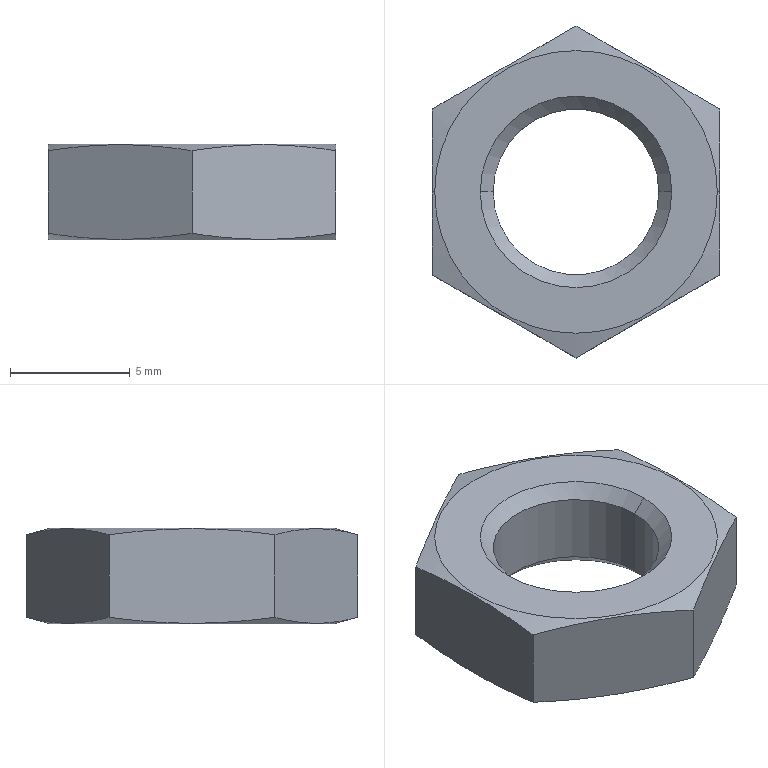Part | SolidWorks | features BaseBody 1 | 1 solid | 18 faces | box 12 x 13.856 x 4 mm | volume 339.344 mm3 | cone 8 | plane 8 | cylinder 2 | commonest cylinder face diameters 6.917 x2
STEP:
#1=CARTESIAN_POINT('',(3.459,0.,0.5415));
#2=VERTEX_POINT('',#1);
#3=CARTESIAN_POINT('',(-3.459,0.,0.5415));
#4=VERTEX_POINT('',#3);
#5=CARTESIAN_POINT('',(0.,0.,0.5415));
#6=DIRECTION('',(0.,0.,-1.));
#7=DIRECTION('',(-1.,0.,0.));
#8=AXIS2_PLACEMENT_3D('',#5,#6,#7);
#9=CIRCLE('',#8,3.459);
#10=EDGE_CURVE('',#2,#4,#9,.T.);
#11=ORIENTED_EDGE('',*,*,#10,.F.);
#12=CARTESIAN_POINT('',(4.,0.,0.));
#13=VERTEX_POINT('',#12);
#14=CARTESIAN_POINT('',(3.459,0.,0.5415));
#15=DIRECTION('',(0.7071,0.,-0.7071));
#16=VECTOR('',#15,1000.);
#17=LINE('',#14,#16);
#18=EDGE_CURVE('',#2,#13,#17,.T.);
#19=ORIENTED_EDGE('',*,*,#18,.T.);
#20=CARTESIAN_POINT('',(-4.,0.,0.));
#21=VERTEX_POINT('',#20);
#22=CARTESIAN_POINT('',(0.,0.,0.));
#23=DIRECTION('',(0.,0.,-1.));
#24=DIRECTION('',(-1.,0.,0.));
#25=AXIS2_PLACEMENT_3D('',#22,#23,#24);
#26=CIRCLE('',#25,4.);
#27=EDGE_CURVE('',#13,#21,#26,.T.);
#28=ORIENTED_EDGE('',*,*,#27,.T.);
#29=CARTESIAN_POINT('',(-3.459,0.,0.5415));
#30=DIRECTION('',(-0.7071,0.,-0.7071));
#31=VECTOR('',#30,1000.);
#32=LINE('',#29,#31);
#33=EDGE_CURVE('',#4,#21,#32,.T.);
#34=ORIENTED_EDGE('',*,*,#33,.F.);
#35=EDGE_LOOP('',(#11,#19,#28,#34));
#36=FACE_OUTER_BOUND('',#35,.T.);
#37=CARTESIAN_POINT('',(0.,0.,0.5415));
#38=DIRECTION('',(0.,0.,-1.));
#39=DIRECTION('',(-1.,0.,0.));
#40=AXIS2_PLACEMENT_3D('',#37,#38,#39);
#41=CONICAL_SURFACE('',#40,3.459,0.7854);
#42=ADVANCED_FACE('',(#36),#41,.F.);
#43=CARTESIAN_POINT('',(3.459,0.,3.459));
#44=VERTEX_POINT('',#43);
#45=CARTESIAN_POINT('',(-3.459,0.,3.459));
#46=VERTEX_POINT('',#45);
#47=CARTESIAN_POINT('',(0.,0.,3.459));
#48=DIRECTION('',(0.,0.,-1.));
#49=DIRECTION('',(-1.,0.,0.));
#50=AXIS2_PLACEMENT_3D('',#47,#48,#49);
#51=CIRCLE('',#50,3.459);
#52=EDGE_CURVE('',#44,#46,#51,.T.);
#53=ORIENTED_EDGE('',*,*,#52,.F.);
#54=CARTESIAN_POINT('',(3.459,0.,0.));
#55=DIRECTION('',(0.,0.,-1.));
#56=VECTOR('',#55,1000.);
#57=LINE('',#54,#56);
#58=EDGE_CURVE('',#44,#2,#57,.T.);
#59=ORIENTED_EDGE('',*,*,#58,.T.);
#60=ORIENTED_EDGE('',*,*,#10,.T.);
#61=CARTESIAN_POINT('',(-3.459,0.,0.));
#62=DIRECTION('',(0.,0.,-1.));
#63=VECTOR('',#62,1000.);
#64=LINE('',#61,#63);
#65=EDGE_CURVE('',#46,#4,#64,.T.);
#66=ORIENTED_EDGE('',*,*,#65,.F.);
#67=EDGE_LOOP('',(#53,#59,#60,#66));
#68=FACE_OUTER_BOUND('',#67,.T.);
#69=CARTESIAN_POINT('',(0.,0.,0.));
#70=DIRECTION('',(0.,0.,-1.));
#71=DIRECTION('',(-1.,0.,0.));
#72=AXIS2_PLACEMENT_3D('',#69,#70,#71);
#73=CYLINDRICAL_SURFACE('',#72,3.459);
#74=ADVANCED_FACE('',(#68),#73,.F.);
#75=CARTESIAN_POINT('',(-5.9,0.,0.));
#76=VERTEX_POINT('',#75);
#77=CARTESIAN_POINT('',(5.9,0.,0.));
#78=VERTEX_POINT('',#77);
#79=CARTESIAN_POINT('',(0.,0.,0.));
#80=DIRECTION('',(0.,0.,-1.));
#81=DIRECTION('',(-1.,0.,0.));
#82=AXIS2_PLACEMENT_3D('',#79,#80,#81);
#83=CIRCLE('',#82,5.9);
#84=EDGE_CURVE('',#76,#78,#83,.T.);
#85=ORIENTED_EDGE('',*,*,#84,.F.);
#86=CARTESIAN_POINT('',(-6.,-0.000000259,0.02686));
#87=VERTEX_POINT('',#86);
#88=CARTESIAN_POINT('',(-5.9,0.,0.));
#89=DIRECTION('',(-0.9659,0.,0.2588));
#90=VECTOR('',#89,1000.);
#91=LINE('',#88,#90);
#92=EDGE_CURVE('',#76,#87,#91,.T.);
#93=ORIENTED_EDGE('',*,*,#92,.T.);
#94=CARTESIAN_POINT('',(-6.,3.464,0.2755));
#95=VERTEX_POINT('',#94);
#96=CARTESIAN_POINT('',(-6.,3.464,0.2755));
#97=CARTESIAN_POINT('',(-6.,2.318,0.122));
#98=CARTESIAN_POINT('',(-6.,1.165,0.02685));
#99=CARTESIAN_POINT('',(-6.,-0.000000259,0.02686));
#100=B_SPLINE_CURVE_WITH_KNOTS('',3,(#96,#97,#98,#99),.UNSPECIFIED.,.F.,.F.,(4,4),(7.335,10.801),.UNSPECIFIED.);
#101=EDGE_CURVE('',#95,#87,#100,.T.);
#102=ORIENTED_EDGE('',*,*,#101,.F.);
#103=CARTESIAN_POINT('',(0.,6.928,0.2755));
#104=VERTEX_POINT('',#103);
#105=CARTESIAN_POINT('',(0.,6.928,0.2755));
#106=CARTESIAN_POINT('',(-0.4983,6.64,0.1984));
#107=CARTESIAN_POINT('',(-0.9989,6.351,0.1355));
#108=CARTESIAN_POINT('',(-2.,5.774,0.04953));
#109=CARTESIAN_POINT('',(-2.499,5.485,0.02679));
#110=CARTESIAN_POINT('',(-3.501,4.907,0.02679));
#111=CARTESIAN_POINT('',(-4.,4.619,0.04953));
#112=CARTESIAN_POINT('',(-5.001,4.041,0.1355));
#113=CARTESIAN_POINT('',(-5.502,3.752,0.1984));
#114=CARTESIAN_POINT('',(-6.,3.464,0.2755));
#115=B_SPLINE_CURVE_WITH_KNOTS('',3,(#105,#106,#107,#108,#109,#110,#111,#112,#113,#114),.UNSPECIFIED.,.F.,.F.,(4,2,2,2,4),(0.0002309,1.732,3.464,5.196,6.928),.UNSPECIFIED.);
#116=EDGE_CURVE('',#104,#95,#115,.T.);
#117=ORIENTED_EDGE('',*,*,#116,.F.);
#118=CARTESIAN_POINT('',(6.,3.464,0.2755));
#119=VERTEX_POINT('',#118);
#120=CARTESIAN_POINT('',(6.,3.464,0.2755));
#121=CARTESIAN_POINT('',(5.502,3.752,0.1984));
#122=CARTESIAN_POINT('',(5.001,4.041,0.1355));
#123=CARTESIAN_POINT('',(4.,4.619,0.04953));
#124=CARTESIAN_POINT('',(3.501,4.907,0.02679));
#125=CARTESIAN_POINT('',(2.499,5.485,0.02679));
#126=CARTESIAN_POINT('',(2.,5.774,0.04953));
#127=CARTESIAN_POINT('',(0.9989,6.351,0.1355));
#128=CARTESIAN_POINT('',(0.4983,6.64,0.1984));
#129=CARTESIAN_POINT('',(0.,6.928,0.2755));
#130=B_SPLINE_CURVE_WITH_KNOTS('',3,(#120,#121,#122,#123,#124,#125,#126,#127,#128,#129),.UNSPECIFIED.,.F.,.F.,(4,2,2,2,4),(0.0002309,1.732,3.464,5.196,6.928),.UNSPECIFIED.);
#131=EDGE_CURVE('',#119,#104,#130,.T.);
#132=ORIENTED_EDGE('',*,*,#131,.F.);
#133=CARTESIAN_POINT('',(6.,0.000000259,0.02686));
#134=VERTEX_POINT('',#133);
#135=CARTESIAN_POINT('',(6.,0.000000259,0.02686));
#136=CARTESIAN_POINT('',(6.,0.5746,0.02679));
#137=CARTESIAN_POINT('',(6.,1.154,0.04948));
#138=CARTESIAN_POINT('',(6.,2.311,0.1354));
#139=CARTESIAN_POINT('',(6.,2.889,0.1984));
#140=CARTESIAN_POINT('',(6.,3.464,0.2755));
#141=B_SPLINE_CURVE_WITH_KNOTS('',3,(#135,#136,#137,#138,#139,#140),.UNSPECIFIED.,.F.,.F.,(4,2,4),(10.801,12.511,14.221),.UNSPECIFIED.);
#142=EDGE_CURVE('',#134,#119,#141,.T.);
#143=ORIENTED_EDGE('',*,*,#142,.F.);
#144=CARTESIAN_POINT('',(5.9,0.,0.));
#145=DIRECTION('',(0.9659,0.,0.2588));
#146=VECTOR('',#145,1000.);
#147=LINE('',#144,#146);
#148=EDGE_CURVE('',#78,#134,#147,.T.);
#149=ORIENTED_EDGE('',*,*,#148,.F.);
#150=EDGE_LOOP('',(#85,#93,#102,#117,#132,#143,#149));
#151=FACE_OUTER_BOUND('',#150,.T.);
#152=CARTESIAN_POINT('',(0.,0.,0.));
#153=DIRECTION('',(0.,0.,1.));
#154=DIRECTION('',(1.,0.,0.));
#155=AXIS2_PLACEMENT_3D('',#152,#153,#154);
#156=CONICAL_SURFACE('',#155,5.9,1.309);
#157=ADVANCED_FACE('',(#151),#156,.T.);
#158=ORIENTED_EDGE('',*,*,#52,.T.);
#159=CARTESIAN_POINT('',(-4.,0.,4.));
#160=VERTEX_POINT('',#159);
#161=CARTESIAN_POINT('',(-4.,0.,4.));
#162=DIRECTION('',(-0.7071,0.,0.7071));
#163=VECTOR('',#162,1000.);
#164=LINE('',#161,#163);
#165=EDGE_CURVE('',#46,#160,#164,.T.);
#166=ORIENTED_EDGE('',*,*,#165,.T.);
#167=CARTESIAN_POINT('',(4.,0.,4.));
#168=VERTEX_POINT('',#167);
#169=CARTESIAN_POINT('',(0.,0.,4.));
#170=DIRECTION('',(0.,0.,-1.));
#171=DIRECTION('',(-1.,0.,0.));
#172=AXIS2_PLACEMENT_3D('',#169,#170,#171);
#173=CIRCLE('',#172,4.);
#174=EDGE_CURVE('',#168,#160,#173,.T.);
#175=ORIENTED_EDGE('',*,*,#174,.F.);
#176=CARTESIAN_POINT('',(4.,0.,4.));
#177=DIRECTION('',(0.7071,0.,0.7071));
#178=VECTOR('',#177,1000.);
#179=LINE('',#176,#178);
#180=EDGE_CURVE('',#44,#168,#179,.T.);
#181=ORIENTED_EDGE('',*,*,#180,.F.);
#182=EDGE_LOOP('',(#158,#166,#175,#181));
#183=FACE_OUTER_BOUND('',#182,.T.);
#184=CARTESIAN_POINT('',(0.,0.,4.));
#185=DIRECTION('',(0.,0.,1.));
#186=DIRECTION('',(1.,0.,0.));
#187=AXIS2_PLACEMENT_3D('',#184,#185,#186);
#188=CONICAL_SURFACE('',#187,4.,0.7854);
#189=ADVANCED_FACE('',(#183),#188,.F.);
#190=CARTESIAN_POINT('',(-5.9,0.,4.));
#191=VERTEX_POINT('',#190);
#192=CARTESIAN_POINT('',(5.9,0.,4.));
#193=VERTEX_POINT('',#192);
#194=CARTESIAN_POINT('',(0.,0.,4.));
#195=DIRECTION('',(0.,0.,-1.));
#196=DIRECTION('',(-1.,0.,0.));
#197=AXIS2_PLACEMENT_3D('',#194,#195,#196);
#198=CIRCLE('',#197,5.9);
#199=EDGE_CURVE('',#191,#193,#198,.T.);
#200=ORIENTED_EDGE('',*,*,#199,.T.);
#201=CARTESIAN_POINT('',(6.,-0.000000259,3.973));
#202=VERTEX_POINT('',#201);
#203=CARTESIAN_POINT('',(13.364,0.,2.));
#204=DIRECTION('',(0.9659,0.,-0.2588));
#205=VECTOR('',#204,1000.);
#206=LINE('',#203,#205);
#207=EDGE_CURVE('',#193,#202,#206,.T.);
#208=ORIENTED_EDGE('',*,*,#207,.T.);
#209=CARTESIAN_POINT('',(6.,3.464,3.724));
#210=VERTEX_POINT('',#209);
#211=CARTESIAN_POINT('',(6.,3.464,3.724));
#212=CARTESIAN_POINT('',(6.,2.318,3.878));
#213=CARTESIAN_POINT('',(6.,1.165,3.973));
#214=CARTESIAN_POINT('',(6.,-0.000000259,3.973));
#215=B_SPLINE_CURVE_WITH_KNOTS('',3,(#211,#212,#213,#214),.UNSPECIFIED.,.F.,.F.,(4,4),(7.335,10.801),.UNSPECIFIED.);
#216=EDGE_CURVE('',#210,#202,#215,.T.);
#217=ORIENTED_EDGE('',*,*,#216,.F.);
#218=CARTESIAN_POINT('',(0.,6.928,3.724));
#219=VERTEX_POINT('',#218);
#220=CARTESIAN_POINT('',(0.,6.928,3.724));
#221=CARTESIAN_POINT('',(0.4983,6.64,3.802));
#222=CARTESIAN_POINT('',(0.9989,6.351,3.865));
#223=CARTESIAN_POINT('',(2.,5.774,3.95));
#224=CARTESIAN_POINT('',(2.499,5.485,3.973));
#225=CARTESIAN_POINT('',(3.501,4.907,3.973));
#226=CARTESIAN_POINT('',(4.,4.619,3.95));
#227=CARTESIAN_POINT('',(5.001,4.041,3.865));
#228=CARTESIAN_POINT('',(5.502,3.752,3.802));
#229=CARTESIAN_POINT('',(6.,3.464,3.724));
#230=B_SPLINE_CURVE_WITH_KNOTS('',3,(#220,#221,#222,#223,#224,#225,#226,#227,#228,#229),.UNSPECIFIED.,.F.,.F.,(4,2,2,2,4),(0.0002309,1.732,3.464,5.196,6.928),.UNSPECIFIED.);
#231=EDGE_CURVE('',#219,#210,#230,.T.);
#232=ORIENTED_EDGE('',*,*,#231,.F.);
#233=CARTESIAN_POINT('',(-6.,3.464,3.724));
#234=VERTEX_POINT('',#233);
#235=CARTESIAN_POINT('',(-6.,3.464,3.724));
#236=CARTESIAN_POINT('',(-5.502,3.752,3.802));
#237=CARTESIAN_POINT('',(-5.001,4.041,3.865));
#238=CARTESIAN_POINT('',(-4.,4.619,3.95));
#239=CARTESIAN_POINT('',(-3.501,4.907,3.973));
#240=CARTESIAN_POINT('',(-2.499,5.485,3.973));
#241=CARTESIAN_POINT('',(-2.,5.774,3.95));
#242=CARTESIAN_POINT('',(-0.9989,6.351,3.865));
#243=CARTESIAN_POINT('',(-0.4983,6.64,3.802));
#244=CARTESIAN_POINT('',(0.,6.928,3.724));
#245=B_SPLINE_CURVE_WITH_KNOTS('',3,(#235,#236,#237,#238,#239,#240,#241,#242,#243,#244),.UNSPECIFIED.,.F.,.F.,(4,2,2,2,4),(0.0002309,1.732,3.464,5.196,6.928),.UNSPECIFIED.);
#246=EDGE_CURVE('',#234,#219,#245,.T.);
#247=ORIENTED_EDGE('',*,*,#246,.F.);
#248=CARTESIAN_POINT('',(-6.,0.000000259,3.973));
#249=VERTEX_POINT('',#248);
#250=CARTESIAN_POINT('',(-6.,0.000000259,3.973));
#251=CARTESIAN_POINT('',(-6.,0.5746,3.973));
#252=CARTESIAN_POINT('',(-6.,1.154,3.951));
#253=CARTESIAN_POINT('',(-6.,2.311,3.865));
#254=CARTESIAN_POINT('',(-6.,2.889,3.802));
#255=CARTESIAN_POINT('',(-6.,3.464,3.724));
#256=B_SPLINE_CURVE_WITH_KNOTS('',3,(#250,#251,#252,#253,#254,#255),.UNSPECIFIED.,.F.,.F.,(4,2,4),(10.801,12.511,14.221),.UNSPECIFIED.);
#257=EDGE_CURVE('',#249,#234,#256,.T.);
#258=ORIENTED_EDGE('',*,*,#257,.F.);
#259=CARTESIAN_POINT('',(-13.364,0.,2.));
#260=DIRECTION('',(-0.9659,0.,-0.2588));
#261=VECTOR('',#260,1000.);
#262=LINE('',#259,#261);
#263=EDGE_CURVE('',#191,#249,#262,.T.);
#264=ORIENTED_EDGE('',*,*,#263,.F.);
#265=EDGE_LOOP('',(#200,#208,#217,#232,#247,#258,#264));
#266=FACE_OUTER_BOUND('',#265,.T.);
#267=CARTESIAN_POINT('',(0.,0.,2.));
#268=DIRECTION('',(0.,0.,-1.));
#269=DIRECTION('',(-1.,0.,0.));
#270=AXIS2_PLACEMENT_3D('',#267,#268,#269);
#271=CONICAL_SURFACE('',#270,13.364,1.309);
#272=ADVANCED_FACE('',(#266),#271,.T.);
#273=ORIENTED_EDGE('',*,*,#207,.F.);
#274=CARTESIAN_POINT('',(0.,0.,4.));
#275=DIRECTION('',(0.,0.,-1.));
#276=DIRECTION('',(-1.,0.,0.));
#277=AXIS2_PLACEMENT_3D('',#274,#275,#276);
#278=CIRCLE('',#277,5.9);
#279=EDGE_CURVE('',#193,#191,#278,.T.);
#280=ORIENTED_EDGE('',*,*,#279,.T.);
#281=ORIENTED_EDGE('',*,*,#263,.T.);
#282=CARTESIAN_POINT('',(-6.,-3.464,3.724));
#283=VERTEX_POINT('',#282);
#284=CARTESIAN_POINT('',(-6.,-3.464,3.724));
#285=CARTESIAN_POINT('',(-6.,-2.318,3.878));
#286=CARTESIAN_POINT('',(-6.,-1.165,3.973));
#287=CARTESIAN_POINT('',(-6.,0.000000259,3.973));
#288=B_SPLINE_CURVE_WITH_KNOTS('',3,(#284,#285,#286,#287),.UNSPECIFIED.,.F.,.F.,(4,4),(7.335,10.801),.UNSPECIFIED.);
#289=EDGE_CURVE('',#283,#249,#288,.T.);
#290=ORIENTED_EDGE('',*,*,#289,.F.);
#291=CARTESIAN_POINT('',(0.,-6.928,3.724));
#292=VERTEX_POINT('',#291);
#293=CARTESIAN_POINT('',(0.,-6.928,3.724));
#294=CARTESIAN_POINT('',(-0.4983,-6.64,3.802));
#295=CARTESIAN_POINT('',(-0.9989,-6.351,3.865));
#296=CARTESIAN_POINT('',(-2.,-5.774,3.95));
#297=CARTESIAN_POINT('',(-2.499,-5.485,3.973));
#298=CARTESIAN_POINT('',(-3.501,-4.907,3.973));
#299=CARTESIAN_POINT('',(-4.,-4.619,3.95));
#300=CARTESIAN_POINT('',(-5.001,-4.041,3.865));
#301=CARTESIAN_POINT('',(-5.502,-3.752,3.802));
#302=CARTESIAN_POINT('',(-6.,-3.464,3.724));
#303=B_SPLINE_CURVE_WITH_KNOTS('',3,(#293,#294,#295,#296,#297,#298,#299,#300,#301,#302),.UNSPECIFIED.,.F.,.F.,(4,2,2,2,4),(0.0002309,1.732,3.464,5.196,6.928),.UNSPECIFIED.);
#304=EDGE_CURVE('',#292,#283,#303,.T.);
#305=ORIENTED_EDGE('',*,*,#304,.F.);
#306=CARTESIAN_POINT('',(6.,-3.464,3.724));
#307=VERTEX_POINT('',#306);
#308=CARTESIAN_POINT('',(6.,-3.464,3.724));
#309=CARTESIAN_POINT('',(5.502,-3.752,3.802));
#310=CARTESIAN_POINT('',(5.001,-4.041,3.865));
#311=CARTESIAN_POINT('',(4.,-4.619,3.95));
#312=CARTESIAN_POINT('',(3.501,-4.907,3.973));
#313=CARTESIAN_POINT('',(2.499,-5.485,3.973));
#314=CARTESIAN_POINT('',(2.,-5.774,3.95));
#315=CARTESIAN_POINT('',(0.9989,-6.351,3.865));
#316=CARTESIAN_POINT('',(0.4983,-6.64,3.802));
#317=CARTESIAN_POINT('',(0.,-6.928,3.724));
#318=B_SPLINE_CURVE_WITH_KNOTS('',3,(#308,#309,#310,#311,#312,#313,#314,#315,#316,#317),.UNSPECIFIED.,.F.,.F.,(4,2,2,2,4),(0.0002309,1.732,3.464,5.196,6.928),.UNSPECIFIED.);
#319=EDGE_CURVE('',#307,#292,#318,.T.);
#320=ORIENTED_EDGE('',*,*,#319,.F.);
#321=CARTESIAN_POINT('',(6.,-0.000000259,3.973));
#322=CARTESIAN_POINT('',(6.,-0.5746,3.973));
#323=CARTESIAN_POINT('',(6.,-1.154,3.951));
#324=CARTESIAN_POINT('',(6.,-2.311,3.865));
#325=CARTESIAN_POINT('',(6.,-2.889,3.802));
#326=CARTESIAN_POINT('',(6.,-3.464,3.724));
#327=B_SPLINE_CURVE_WITH_KNOTS('',3,(#321,#322,#323,#324,#325,#326),.UNSPECIFIED.,.F.,.F.,(4,2,4),(10.801,12.511,14.221),.UNSPECIFIED.);
#328=EDGE_CURVE('',#202,#307,#327,.T.);
#329=ORIENTED_EDGE('',*,*,#328,.F.);
#330=EDGE_LOOP('',(#273,#280,#281,#290,#305,#320,#329));
#331=FACE_OUTER_BOUND('',#330,.T.);
#332=CARTESIAN_POINT('',(0.,0.,2.));
#333=DIRECTION('',(0.,0.,-1.));
#334=DIRECTION('',(-1.,0.,0.));
#335=AXIS2_PLACEMENT_3D('',#332,#333,#334);
#336=CONICAL_SURFACE('',#335,13.364,1.309);
#337=ADVANCED_FACE('',(#331),#336,.T.);
#338=ORIENTED_EDGE('',*,*,#174,.T.);
#339=CARTESIAN_POINT('',(0.,0.,4.));
#340=DIRECTION('',(0.,0.,-1.));
#341=DIRECTION('',(-1.,0.,0.));
#342=AXIS2_PLACEMENT_3D('',#339,#340,#341);
#343=CIRCLE('',#342,4.);
#344=EDGE_CURVE('',#160,#168,#343,.T.);
#345=ORIENTED_EDGE('',*,*,#344,.T.);
#346=EDGE_LOOP('',(#338,#345));
#347=FACE_BOUND('',#346,.T.);
#348=ORIENTED_EDGE('',*,*,#199,.F.);
#349=ORIENTED_EDGE('',*,*,#279,.F.);
#350=EDGE_LOOP('',(#348,#349));
#351=FACE_OUTER_BOUND('',#350,.T.);
#352=CARTESIAN_POINT('',(0.,5.9,4.));
#353=DIRECTION('',(0.,0.,1.));
#354=DIRECTION('',(1.,0.,0.));
#355=AXIS2_PLACEMENT_3D('',#352,#353,#354);
#356=PLANE('',#355);
#357=ADVANCED_FACE('',(#347,#351),#356,.T.);
#358=ORIENTED_EDGE('',*,*,#289,.T.);
#359=ORIENTED_EDGE('',*,*,#257,.T.);
#360=CARTESIAN_POINT('',(-6.,3.464,3.724));
#361=DIRECTION('',(0.,0.,-1.));
#362=VECTOR('',#361,1000.);
#363=LINE('',#360,#362);
#364=EDGE_CURVE('',#234,#95,#363,.T.);
#365=ORIENTED_EDGE('',*,*,#364,.T.);
#366=ORIENTED_EDGE('',*,*,#101,.T.);
#367=CARTESIAN_POINT('',(-6.,-3.464,0.2755));
#368=VERTEX_POINT('',#367);
#369=CARTESIAN_POINT('',(-6.,-0.000000259,0.02686));
#370=CARTESIAN_POINT('',(-6.,-0.5746,0.02679));
#371=CARTESIAN_POINT('',(-6.,-1.154,0.04948));
#372=CARTESIAN_POINT('',(-6.,-2.311,0.1354));
#373=CARTESIAN_POINT('',(-6.,-2.889,0.1984));
#374=CARTESIAN_POINT('',(-6.,-3.464,0.2755));
#375=B_SPLINE_CURVE_WITH_KNOTS('',3,(#369,#370,#371,#372,#373,#374),.UNSPECIFIED.,.F.,.F.,(4,2,4),(10.801,12.511,14.221),.UNSPECIFIED.);
#376=EDGE_CURVE('',#87,#368,#375,.T.);
#377=ORIENTED_EDGE('',*,*,#376,.T.);
#378=CARTESIAN_POINT('',(-6.,-3.464,3.724));
#379=DIRECTION('',(0.,0.,-1.));
#380=VECTOR('',#379,1000.);
#381=LINE('',#378,#380);
#382=EDGE_CURVE('',#283,#368,#381,.T.);
#383=ORIENTED_EDGE('',*,*,#382,.F.);
#384=EDGE_LOOP('',(#358,#359,#365,#366,#377,#383));
#385=FACE_OUTER_BOUND('',#384,.T.);
#386=CARTESIAN_POINT('',(-6.,3.464,4.));
#387=DIRECTION('',(1.,0.,0.));
#388=DIRECTION('',(0.,0.,-1.));
#389=AXIS2_PLACEMENT_3D('',#386,#387,#388);
#390=PLANE('',#389);
#391=ADVANCED_FACE('',(#385),#390,.F.);
#392=ORIENTED_EDGE('',*,*,#304,.T.);
#393=ORIENTED_EDGE('',*,*,#382,.T.);
#394=CARTESIAN_POINT('',(0.,-6.928,0.2755));
#395=VERTEX_POINT('',#394);
#396=CARTESIAN_POINT('',(-6.,-3.464,0.2755));
#397=CARTESIAN_POINT('',(-5.502,-3.752,0.1984));
#398=CARTESIAN_POINT('',(-5.001,-4.041,0.1355));
#399=CARTESIAN_POINT('',(-4.,-4.619,0.04953));
#400=CARTESIAN_POINT('',(-3.501,-4.907,0.02679));
#401=CARTESIAN_POINT('',(-2.499,-5.485,0.02679));
#402=CARTESIAN_POINT('',(-2.,-5.774,0.04953));
#403=CARTESIAN_POINT('',(-0.9989,-6.351,0.1355));
#404=CARTESIAN_POINT('',(-0.4983,-6.64,0.1984));
#405=CARTESIAN_POINT('',(0.,-6.928,0.2755));
#406=B_SPLINE_CURVE_WITH_KNOTS('',3,(#396,#397,#398,#399,#400,#401,#402,#403,#404,#405),.UNSPECIFIED.,.F.,.F.,(4,2,2,2,4),(0.0002309,1.732,3.464,5.196,6.928),.UNSPECIFIED.);
#407=EDGE_CURVE('',#368,#395,#406,.T.);
#408=ORIENTED_EDGE('',*,*,#407,.T.);
#409=CARTESIAN_POINT('',(0.,-6.928,3.724));
#410=DIRECTION('',(0.,0.,-1.));
#411=VECTOR('',#410,1000.);
#412=LINE('',#409,#411);
#413=EDGE_CURVE('',#292,#395,#412,.T.);
#414=ORIENTED_EDGE('',*,*,#413,.F.);
#415=EDGE_LOOP('',(#392,#393,#408,#414));
#416=FACE_OUTER_BOUND('',#415,.T.);
#417=CARTESIAN_POINT('',(-6.,-3.464,4.));
#418=DIRECTION('',(0.5,0.866,0.));
#419=DIRECTION('',(-0.866,0.5,0.));
#420=AXIS2_PLACEMENT_3D('',#417,#418,#419);
#421=PLANE('',#420);
#422=ADVANCED_FACE('',(#416),#421,.F.);
#423=ORIENTED_EDGE('',*,*,#319,.T.);
#424=ORIENTED_EDGE('',*,*,#413,.T.);
#425=CARTESIAN_POINT('',(6.,-3.464,0.2755));
#426=VERTEX_POINT('',#425);
#427=CARTESIAN_POINT('',(0.,-6.928,0.2755));
#428=CARTESIAN_POINT('',(0.4983,-6.64,0.1984));
#429=CARTESIAN_POINT('',(0.9989,-6.351,0.1355));
#430=CARTESIAN_POINT('',(2.,-5.774,0.04953));
#431=CARTESIAN_POINT('',(2.499,-5.485,0.02679));
#432=CARTESIAN_POINT('',(3.501,-4.907,0.02679));
#433=CARTESIAN_POINT('',(4.,-4.619,0.04953));
#434=CARTESIAN_POINT('',(5.001,-4.041,0.1355));
#435=CARTESIAN_POINT('',(5.502,-3.752,0.1984));
#436=CARTESIAN_POINT('',(6.,-3.464,0.2755));
#437=B_SPLINE_CURVE_WITH_KNOTS('',3,(#427,#428,#429,#430,#431,#432,#433,#434,#435,#436),.UNSPECIFIED.,.F.,.F.,(4,2,2,2,4),(0.0002309,1.732,3.464,5.196,6.928),.UNSPECIFIED.);
#438=EDGE_CURVE('',#395,#426,#437,.T.);
#439=ORIENTED_EDGE('',*,*,#438,.T.);
#440=CARTESIAN_POINT('',(6.,-3.464,3.724));
#441=DIRECTION('',(0.,0.,-1.));
#442=VECTOR('',#441,1000.);
#443=LINE('',#440,#442);
#444=EDGE_CURVE('',#307,#426,#443,.T.);
#445=ORIENTED_EDGE('',*,*,#444,.F.);
#446=EDGE_LOOP('',(#423,#424,#439,#445));
#447=FACE_OUTER_BOUND('',#446,.T.);
#448=CARTESIAN_POINT('',(0.,-6.928,4.));
#449=DIRECTION('',(-0.5,0.866,0.));
#450=DIRECTION('',(-0.866,-0.5,0.));
#451=AXIS2_PLACEMENT_3D('',#448,#449,#450);
#452=PLANE('',#451);
#453=ADVANCED_FACE('',(#447),#452,.F.);
#454=ORIENTED_EDGE('',*,*,#216,.T.);
#455=ORIENTED_EDGE('',*,*,#328,.T.);
#456=ORIENTED_EDGE('',*,*,#444,.T.);
#457=CARTESIAN_POINT('',(6.,-3.464,0.2755));
#458=CARTESIAN_POINT('',(6.,-2.318,0.122));
#459=CARTESIAN_POINT('',(6.,-1.165,0.02685));
#460=CARTESIAN_POINT('',(6.,0.000000259,0.02686));
#461=B_SPLINE_CURVE_WITH_KNOTS('',3,(#457,#458,#459,#460),.UNSPECIFIED.,.F.,.F.,(4,4),(7.335,10.801),.UNSPECIFIED.);
#462=EDGE_CURVE('',#426,#134,#461,.T.);
#463=ORIENTED_EDGE('',*,*,#462,.T.);
#464=ORIENTED_EDGE('',*,*,#142,.T.);
#465=CARTESIAN_POINT('',(6.,3.464,3.724));
#466=DIRECTION('',(0.,0.,-1.));
#467=VECTOR('',#466,1000.);
#468=LINE('',#465,#467);
#469=EDGE_CURVE('',#210,#119,#468,.T.);
#470=ORIENTED_EDGE('',*,*,#469,.F.);
#471=EDGE_LOOP('',(#454,#455,#456,#463,#464,#470));
#472=FACE_OUTER_BOUND('',#471,.T.);
#473=CARTESIAN_POINT('',(6.,-3.464,4.));
#474=DIRECTION('',(-1.,0.,0.));
#475=DIRECTION('',(0.,0.,1.));
#476=AXIS2_PLACEMENT_3D('',#473,#474,#475);
#477=PLANE('',#476);
#478=ADVANCED_FACE('',(#472),#477,.F.);
#479=ORIENTED_EDGE('',*,*,#231,.T.);
#480=ORIENTED_EDGE('',*,*,#469,.T.);
#481=ORIENTED_EDGE('',*,*,#131,.T.);
#482=CARTESIAN_POINT('',(0.,6.928,3.724));
#483=DIRECTION('',(0.,0.,-1.));
#484=VECTOR('',#483,1000.);
#485=LINE('',#482,#484);
#486=EDGE_CURVE('',#219,#104,#485,.T.);
#487=ORIENTED_EDGE('',*,*,#486,.F.);
#488=EDGE_LOOP('',(#479,#480,#481,#487));
#489=FACE_OUTER_BOUND('',#488,.T.);
#490=CARTESIAN_POINT('',(6.,3.464,4.));
#491=DIRECTION('',(-0.5,-0.866,0.));
#492=DIRECTION('',(0.866,-0.5,0.));
#493=AXIS2_PLACEMENT_3D('',#490,#491,#492);
#494=PLANE('',#493);
#495=ADVANCED_FACE('',(#489),#494,.F.);
#496=ORIENTED_EDGE('',*,*,#246,.T.);
#497=ORIENTED_EDGE('',*,*,#486,.T.);
#498=ORIENTED_EDGE('',*,*,#116,.T.);
#499=ORIENTED_EDGE('',*,*,#364,.F.);
#500=EDGE_LOOP('',(#496,#497,#498,#499));
#501=FACE_OUTER_BOUND('',#500,.T.);
#502=CARTESIAN_POINT('',(0.,6.928,4.));
#503=DIRECTION('',(0.5,-0.866,0.));
#504=DIRECTION('',(0.866,0.5,0.));
#505=AXIS2_PLACEMENT_3D('',#502,#503,#504);
#506=PLANE('',#505);
#507=ADVANCED_FACE('',(#501),#506,.F.);
#508=ORIENTED_EDGE('',*,*,#165,.F.);
#509=CARTESIAN_POINT('',(0.,0.,3.459));
#510=DIRECTION('',(0.,0.,-1.));
#511=DIRECTION('',(-1.,0.,0.));
#512=AXIS2_PLACEMENT_3D('',#509,#510,#511);
#513=CIRCLE('',#512,3.459);
#514=EDGE_CURVE('',#46,#44,#513,.T.);
#515=ORIENTED_EDGE('',*,*,#514,.T.);
#516=ORIENTED_EDGE('',*,*,#180,.T.);
#517=ORIENTED_EDGE('',*,*,#344,.F.);
#518=EDGE_LOOP('',(#508,#515,#516,#517));
#519=FACE_OUTER_BOUND('',#518,.T.);
#520=CARTESIAN_POINT('',(0.,0.,4.));
#521=DIRECTION('',(0.,0.,1.));
#522=DIRECTION('',(1.,0.,0.));
#523=AXIS2_PLACEMENT_3D('',#520,#521,#522);
#524=CONICAL_SURFACE('',#523,4.,0.7854);
#525=ADVANCED_FACE('',(#519),#524,.F.);
#526=ORIENTED_EDGE('',*,*,#92,.F.);
#527=CARTESIAN_POINT('',(0.,0.,0.));
#528=DIRECTION('',(0.,0.,-1.));
#529=DIRECTION('',(-1.,0.,0.));
#530=AXIS2_PLACEMENT_3D('',#527,#528,#529);
#531=CIRCLE('',#530,5.9);
#532=EDGE_CURVE('',#78,#76,#531,.T.);
#533=ORIENTED_EDGE('',*,*,#532,.F.);
#534=ORIENTED_EDGE('',*,*,#148,.T.);
#535=ORIENTED_EDGE('',*,*,#462,.F.);
#536=ORIENTED_EDGE('',*,*,#438,.F.);
#537=ORIENTED_EDGE('',*,*,#407,.F.);
#538=ORIENTED_EDGE('',*,*,#376,.F.);
#539=EDGE_LOOP('',(#526,#533,#534,#535,#536,#537,#538));
#540=FACE_OUTER_BOUND('',#539,.T.);
#541=CARTESIAN_POINT('',(0.,0.,0.));
#542=DIRECTION('',(0.,0.,1.));
#543=DIRECTION('',(1.,0.,0.));
#544=AXIS2_PLACEMENT_3D('',#541,#542,#543);
#545=CONICAL_SURFACE('',#544,5.9,1.309);
#546=ADVANCED_FACE('',(#540),#545,.T.);
#547=ORIENTED_EDGE('',*,*,#58,.F.);
#548=ORIENTED_EDGE('',*,*,#514,.F.);
#549=ORIENTED_EDGE('',*,*,#65,.T.);
#550=CARTESIAN_POINT('',(0.,0.,0.5415));
#551=DIRECTION('',(0.,0.,-1.));
#552=DIRECTION('',(-1.,0.,0.));
#553=AXIS2_PLACEMENT_3D('',#550,#551,#552);
#554=CIRCLE('',#553,3.459);
#555=EDGE_CURVE('',#4,#2,#554,.T.);
#556=ORIENTED_EDGE('',*,*,#555,.T.);
#557=EDGE_LOOP('',(#547,#548,#549,#556));
#558=FACE_OUTER_BOUND('',#557,.T.);
#559=CARTESIAN_POINT('',(0.,0.,0.));
#560=DIRECTION('',(0.,0.,-1.));
#561=DIRECTION('',(-1.,0.,0.));
#562=AXIS2_PLACEMENT_3D('',#559,#560,#561);
#563=CYLINDRICAL_SURFACE('',#562,3.459);
#564=ADVANCED_FACE('',(#558),#563,.F.);
#565=ORIENTED_EDGE('',*,*,#532,.T.);
#566=ORIENTED_EDGE('',*,*,#84,.T.);
#567=EDGE_LOOP('',(#565,#566));
#568=FACE_OUTER_BOUND('',#567,.T.);
#569=CARTESIAN_POINT('',(0.,0.,0.));
#570=DIRECTION('',(0.,0.,-1.));
#571=DIRECTION('',(-1.,0.,0.));
#572=AXIS2_PLACEMENT_3D('',#569,#570,#571);
#573=CIRCLE('',#572,4.);
#574=EDGE_CURVE('',#21,#13,#573,.T.);
#575=ORIENTED_EDGE('',*,*,#574,.F.);
#576=ORIENTED_EDGE('',*,*,#27,.F.);
#577=EDGE_LOOP('',(#575,#576));
#578=FACE_BOUND('',#577,.T.);
#579=CARTESIAN_POINT('',(0.,4.,0.));
#580=DIRECTION('',(0.,0.,-1.));
#581=DIRECTION('',(-1.,0.,0.));
#582=AXIS2_PLACEMENT_3D('',#579,#580,#581);
#583=PLANE('',#582);
#584=ADVANCED_FACE('',(#568,#578),#583,.T.);
#585=ORIENTED_EDGE('',*,*,#18,.F.);
#586=ORIENTED_EDGE('',*,*,#555,.F.);
#587=ORIENTED_EDGE('',*,*,#33,.T.);
#588=ORIENTED_EDGE('',*,*,#574,.T.);
#589=EDGE_LOOP('',(#585,#586,#587,#588));
#590=FACE_OUTER_BOUND('',#589,.T.);
#591=CARTESIAN_POINT('',(0.,0.,0.5415));
#592=DIRECTION('',(0.,0.,-1.));
#593=DIRECTION('',(-1.,0.,0.));
#594=AXIS2_PLACEMENT_3D('',#591,#592,#593);
#595=CONICAL_SURFACE('',#594,3.459,0.7854);
#596=ADVANCED_FACE('',(#590),#595,.F.);
#597=CLOSED_SHELL('',(#42,#74,#157,#189,#272,#337,#357,#391,#422,#453,#478,#495,#507,#525,#546,#564,#584,#596));
#598=MANIFOLD_SOLID_BREP('',#597);
#599=CARTESIAN_POINT('',(0.,0.,0.));
#600=DIRECTION('',(0.,0.,1.));
#601=DIRECTION('',(1.,0.,0.));
#602=AXIS2_PLACEMENT_3D('',#599,#600,#601);
#603=(LENGTH_UNIT()NAMED_UNIT(*)SI_UNIT(.MILLI.,.METRE.));
#604=UNCERTAINTY_MEASURE_WITH_UNIT(LENGTH_MEASURE(0.00001),#603,'','');
#605=(NAMED_UNIT(*)PLANE_ANGLE_UNIT()SI_UNIT($,.RADIAN.));
#606=(NAMED_UNIT(*)SI_UNIT($,.STERADIAN.)SOLID_ANGLE_UNIT());
#607=(GEOMETRIC_REPRESENTATION_CONTEXT(3)GLOBAL_UNCERTAINTY_ASSIGNED_CONTEXT((#604))GLOBAL_UNIT_ASSIGNED_CONTEXT((#603,#605,#606))REPRESENTATION_CONTEXT('',''));
#608=ADVANCED_BREP_SHAPE_REPRESENTATION('',(#598,#602),#607);